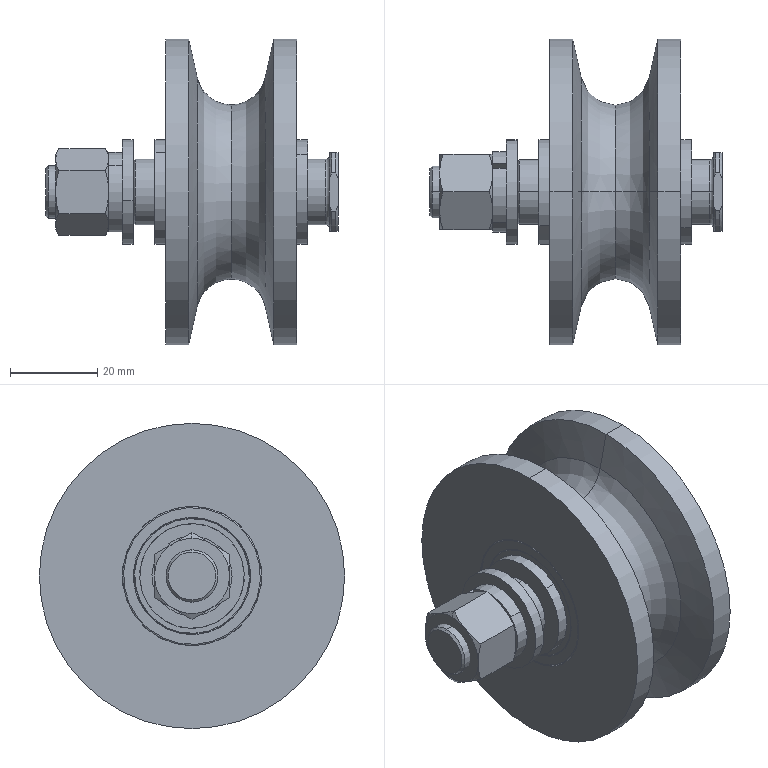Part | SolidWorks | 39 solids | 494 faces | box 67 x 70 x 70 mm | volume 76949 mm3 | cylinder 178 | sphere 120 | plane 102 | torus 52 | cone 42 | commonest cylinder face diameters 22.65 x54 24.35 x54 15 x10 18.778 x8 20.667 x8 26.333 x8